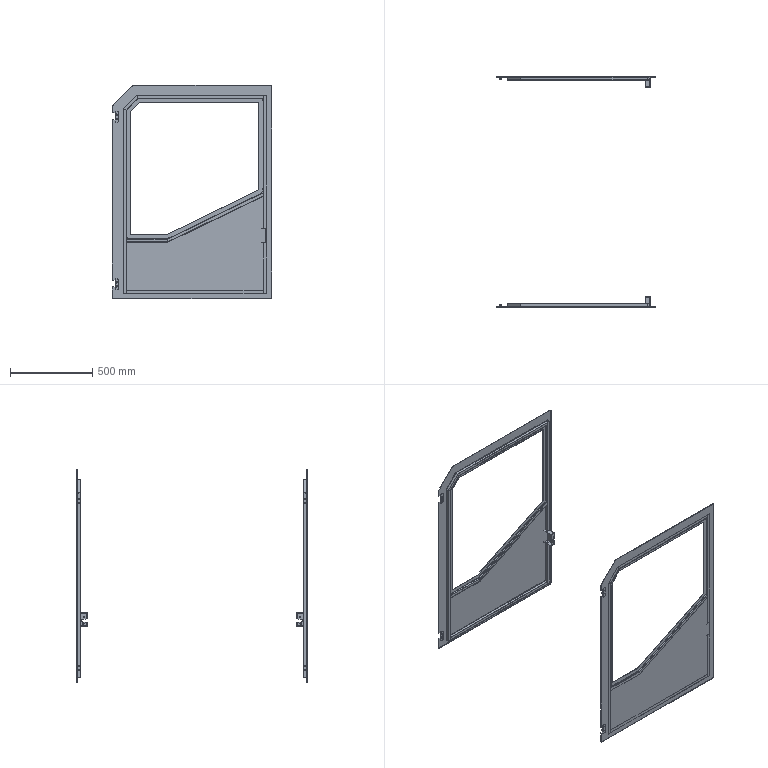Part | NX | features BREP 24 | 38 solids | 724 faces | volume 4247420 mm3 | plane 428 | cylinder 160 | cone 75 | spline 31 | torus 16 | sphere 14 | commonest cylinder face diameters 10 x36 5 x22 7.4 x16 8 x16 10.4 x16 6 x8